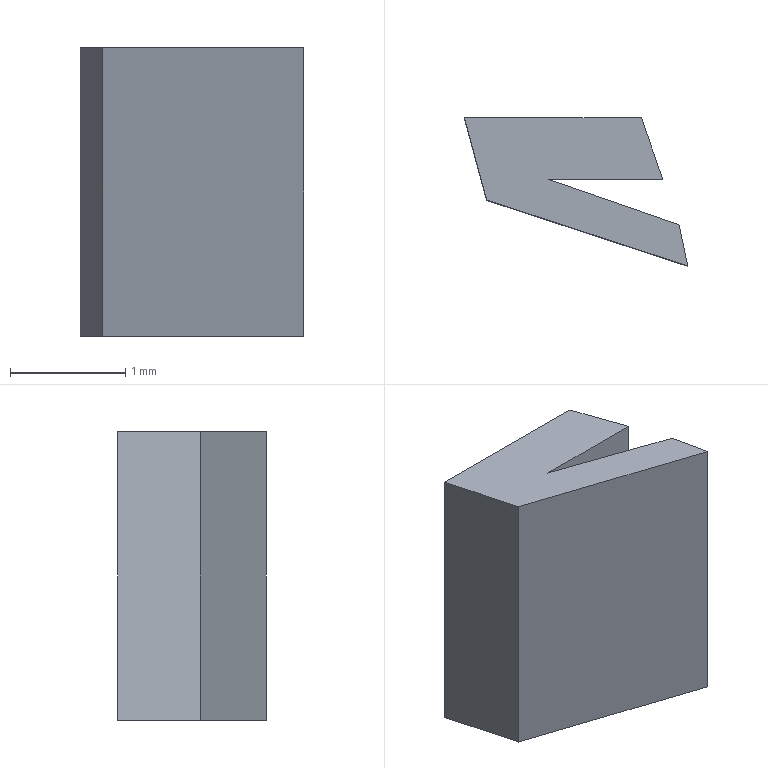Part | STEP file | lll_id1086_x_t | 1 solid | 9 faces | box 1.938 x 1.285 x 2.5 mm | volume 3.455 mm3 | plane 9
STEP:
#1=CARTESIAN_POINT('',(385.109,-124.499,2.35));
#2=VERTEX_POINT('',#1);
#3=CARTESIAN_POINT('',(385.184,-124.857,2.35));
#4=VERTEX_POINT('',#3);
#5=CARTESIAN_POINT('',(385.109,-124.499,2.35));
#6=DIRECTION('',(0.2057,-0.9786,0.));
#7=VECTOR('',#6,1.);
#8=LINE('',#5,#7);
#9=EDGE_CURVE('',#2,#4,#8,.T.);
#10=ORIENTED_EDGE('',*,*,#9,.T.);
#11=CARTESIAN_POINT('',(385.184,-124.857,-0.15));
#12=VERTEX_POINT('',#11);
#13=CARTESIAN_POINT('',(385.184,-124.857,-0.15));
#14=DIRECTION('',(0.,0.,1.));
#15=VECTOR('',#14,1.);
#16=LINE('',#13,#15);
#17=EDGE_CURVE('',#12,#4,#16,.T.);
#18=ORIENTED_EDGE('',*,*,#17,.F.);
#19=CARTESIAN_POINT('',(385.109,-124.499,-0.15));
#20=VERTEX_POINT('',#19);
#21=CARTESIAN_POINT('',(385.109,-124.499,-0.15));
#22=DIRECTION('',(0.2057,-0.9786,0.));
#23=VECTOR('',#22,1.);
#24=LINE('',#21,#23);
#25=EDGE_CURVE('',#20,#12,#24,.T.);
#26=ORIENTED_EDGE('',*,*,#25,.F.);
#27=CARTESIAN_POINT('',(385.109,-124.499,-0.15));
#28=DIRECTION('',(0.,0.,1.));
#29=VECTOR('',#28,1.);
#30=LINE('',#27,#29);
#31=EDGE_CURVE('',#20,#2,#30,.T.);
#32=ORIENTED_EDGE('',*,*,#31,.T.);
#33=EDGE_LOOP('',(#10,#18,#26,#32));
#34=FACE_OUTER_BOUND('',#33,.T.);
#35=CARTESIAN_POINT('',(385.109,-124.499,-0.15));
#36=DIRECTION('',(-0.9786,-0.2057,0.));
#37=DIRECTION('',(-0.2057,0.9786,0.));
#38=AXIS2_PLACEMENT_3D('',#35,#36,#37);
#39=PLANE('',#38);
#40=ADVANCED_FACE('',(#34),#39,.F.);
#41=CARTESIAN_POINT('',(383.439,-124.285,2.35));
#42=VERTEX_POINT('',#41);
#43=CARTESIAN_POINT('',(385.184,-124.857,2.35));
#44=DIRECTION('',(-0.9503,0.3113,0.));
#45=VECTOR('',#44,1.);
#46=LINE('',#43,#45);
#47=EDGE_CURVE('',#4,#42,#46,.T.);
#48=ORIENTED_EDGE('',*,*,#47,.T.);
#49=CARTESIAN_POINT('',(383.439,-124.285,-0.15));
#50=VERTEX_POINT('',#49);
#51=CARTESIAN_POINT('',(383.439,-124.285,-0.15));
#52=DIRECTION('',(0.,0.,1.));
#53=VECTOR('',#52,1.);
#54=LINE('',#51,#53);
#55=EDGE_CURVE('',#50,#42,#54,.T.);
#56=ORIENTED_EDGE('',*,*,#55,.F.);
#57=CARTESIAN_POINT('',(385.184,-124.857,-0.15));
#58=DIRECTION('',(-0.9503,0.3113,0.));
#59=VECTOR('',#58,1.);
#60=LINE('',#57,#59);
#61=EDGE_CURVE('',#12,#50,#60,.T.);
#62=ORIENTED_EDGE('',*,*,#61,.F.);
#63=ORIENTED_EDGE('',*,*,#17,.T.);
#64=EDGE_LOOP('',(#48,#56,#62,#63));
#65=FACE_OUTER_BOUND('',#64,.T.);
#66=CARTESIAN_POINT('',(385.184,-124.857,-0.15));
#67=DIRECTION('',(0.3113,0.9503,0.));
#68=DIRECTION('',(0.9503,-0.3113,0.));
#69=AXIS2_PLACEMENT_3D('',#66,#67,#68);
#70=PLANE('',#69);
#71=ADVANCED_FACE('',(#65),#70,.F.);
#72=CARTESIAN_POINT('',(383.246,-123.572,2.35));
#73=VERTEX_POINT('',#72);
#74=CARTESIAN_POINT('',(383.439,-124.285,2.35));
#75=DIRECTION('',(-0.261,0.9653,0.));
#76=VECTOR('',#75,1.);
#77=LINE('',#74,#76);
#78=EDGE_CURVE('',#42,#73,#77,.T.);
#79=ORIENTED_EDGE('',*,*,#78,.T.);
#80=CARTESIAN_POINT('',(383.246,-123.572,-0.15));
#81=VERTEX_POINT('',#80);
#82=CARTESIAN_POINT('',(383.246,-123.572,-0.15));
#83=DIRECTION('',(0.,0.,1.));
#84=VECTOR('',#83,1.);
#85=LINE('',#82,#84);
#86=EDGE_CURVE('',#81,#73,#85,.T.);
#87=ORIENTED_EDGE('',*,*,#86,.F.);
#88=CARTESIAN_POINT('',(383.439,-124.285,-0.15));
#89=DIRECTION('',(-0.261,0.9653,0.));
#90=VECTOR('',#89,1.);
#91=LINE('',#88,#90);
#92=EDGE_CURVE('',#50,#81,#91,.T.);
#93=ORIENTED_EDGE('',*,*,#92,.F.);
#94=ORIENTED_EDGE('',*,*,#55,.T.);
#95=EDGE_LOOP('',(#79,#87,#93,#94));
#96=FACE_OUTER_BOUND('',#95,.T.);
#97=CARTESIAN_POINT('',(383.439,-124.285,-0.15));
#98=DIRECTION('',(0.9653,0.261,0.));
#99=DIRECTION('',(0.261,-0.9653,0.));
#100=AXIS2_PLACEMENT_3D('',#97,#98,#99);
#101=PLANE('',#100);
#102=ADVANCED_FACE('',(#96),#101,.F.);
#103=CARTESIAN_POINT('',(384.782,-123.572,2.35));
#104=VERTEX_POINT('',#103);
#105=CARTESIAN_POINT('',(383.246,-123.572,2.35));
#106=DIRECTION('',(1.,0.,0.));
#107=VECTOR('',#106,1.);
#108=LINE('',#105,#107);
#109=EDGE_CURVE('',#73,#104,#108,.T.);
#110=ORIENTED_EDGE('',*,*,#109,.T.);
#111=CARTESIAN_POINT('',(384.782,-123.572,-0.15));
#112=VERTEX_POINT('',#111);
#113=CARTESIAN_POINT('',(384.782,-123.572,-0.15));
#114=DIRECTION('',(0.,0.,1.));
#115=VECTOR('',#114,1.);
#116=LINE('',#113,#115);
#117=EDGE_CURVE('',#112,#104,#116,.T.);
#118=ORIENTED_EDGE('',*,*,#117,.F.);
#119=CARTESIAN_POINT('',(383.246,-123.572,-0.15));
#120=DIRECTION('',(1.,0.,0.));
#121=VECTOR('',#120,1.);
#122=LINE('',#119,#121);
#123=EDGE_CURVE('',#81,#112,#122,.T.);
#124=ORIENTED_EDGE('',*,*,#123,.F.);
#125=ORIENTED_EDGE('',*,*,#86,.T.);
#126=EDGE_LOOP('',(#110,#118,#124,#125));
#127=FACE_OUTER_BOUND('',#126,.T.);
#128=CARTESIAN_POINT('',(383.246,-123.572,-0.15));
#129=DIRECTION('',(0.,-1.,0.));
#130=DIRECTION('',(0.,0.,-1.));
#131=AXIS2_PLACEMENT_3D('',#128,#129,#130);
#132=PLANE('',#131);
#133=ADVANCED_FACE('',(#127),#132,.F.);
#134=CARTESIAN_POINT('',(384.969,-124.107,2.35));
#135=VERTEX_POINT('',#134);
#136=CARTESIAN_POINT('',(384.782,-123.572,2.35));
#137=DIRECTION('',(0.3299,-0.944,0.));
#138=VECTOR('',#137,1.);
#139=LINE('',#136,#138);
#140=EDGE_CURVE('',#104,#135,#139,.T.);
#141=ORIENTED_EDGE('',*,*,#140,.T.);
#142=CARTESIAN_POINT('',(384.969,-124.107,-0.15));
#143=VERTEX_POINT('',#142);
#144=CARTESIAN_POINT('',(384.969,-124.107,-0.15));
#145=DIRECTION('',(0.,0.,1.));
#146=VECTOR('',#145,1.);
#147=LINE('',#144,#146);
#148=EDGE_CURVE('',#143,#135,#147,.T.);
#149=ORIENTED_EDGE('',*,*,#148,.F.);
#150=CARTESIAN_POINT('',(384.782,-123.572,-0.15));
#151=DIRECTION('',(0.3299,-0.944,0.));
#152=VECTOR('',#151,1.);
#153=LINE('',#150,#152);
#154=EDGE_CURVE('',#112,#143,#153,.T.);
#155=ORIENTED_EDGE('',*,*,#154,.F.);
#156=ORIENTED_EDGE('',*,*,#117,.T.);
#157=EDGE_LOOP('',(#141,#149,#155,#156));
#158=FACE_OUTER_BOUND('',#157,.T.);
#159=CARTESIAN_POINT('',(384.782,-123.572,-0.15));
#160=DIRECTION('',(-0.944,-0.3299,0.));
#161=DIRECTION('',(-0.3299,0.944,0.));
#162=AXIS2_PLACEMENT_3D('',#159,#160,#161);
#163=PLANE('',#162);
#164=ADVANCED_FACE('',(#158),#163,.F.);
#165=CARTESIAN_POINT('',(383.975,-124.107,2.35));
#166=VERTEX_POINT('',#165);
#167=CARTESIAN_POINT('',(384.969,-124.107,2.35));
#168=DIRECTION('',(-1.,0.,0.));
#169=VECTOR('',#168,1.);
#170=LINE('',#167,#169);
#171=EDGE_CURVE('',#135,#166,#170,.T.);
#172=ORIENTED_EDGE('',*,*,#171,.T.);
#173=CARTESIAN_POINT('',(383.975,-124.107,-0.15));
#174=VERTEX_POINT('',#173);
#175=CARTESIAN_POINT('',(383.975,-124.107,-0.15));
#176=DIRECTION('',(0.,0.,1.));
#177=VECTOR('',#176,1.);
#178=LINE('',#175,#177);
#179=EDGE_CURVE('',#174,#166,#178,.T.);
#180=ORIENTED_EDGE('',*,*,#179,.F.);
#181=CARTESIAN_POINT('',(384.969,-124.107,-0.15));
#182=DIRECTION('',(-1.,0.,0.));
#183=VECTOR('',#182,1.);
#184=LINE('',#181,#183);
#185=EDGE_CURVE('',#143,#174,#184,.T.);
#186=ORIENTED_EDGE('',*,*,#185,.F.);
#187=ORIENTED_EDGE('',*,*,#148,.T.);
#188=EDGE_LOOP('',(#172,#180,#186,#187));
#189=FACE_OUTER_BOUND('',#188,.T.);
#190=CARTESIAN_POINT('',(384.969,-124.107,-0.15));
#191=DIRECTION('',(0.,1.,0.));
#192=DIRECTION('',(0.,0.,1.));
#193=AXIS2_PLACEMENT_3D('',#190,#191,#192);
#194=PLANE('',#193);
#195=ADVANCED_FACE('',(#189),#194,.F.);
#196=CARTESIAN_POINT('',(383.975,-124.107,2.35));
#197=DIRECTION('',(0.9449,-0.3274,0.));
#198=VECTOR('',#197,1.);
#199=LINE('',#196,#198);
#200=EDGE_CURVE('',#166,#2,#199,.T.);
#201=ORIENTED_EDGE('',*,*,#200,.T.);
#202=ORIENTED_EDGE('',*,*,#31,.F.);
#203=CARTESIAN_POINT('',(383.975,-124.107,-0.15));
#204=DIRECTION('',(0.9449,-0.3274,0.));
#205=VECTOR('',#204,1.);
#206=LINE('',#203,#205);
#207=EDGE_CURVE('',#174,#20,#206,.T.);
#208=ORIENTED_EDGE('',*,*,#207,.F.);
#209=ORIENTED_EDGE('',*,*,#179,.T.);
#210=EDGE_LOOP('',(#201,#202,#208,#209));
#211=FACE_OUTER_BOUND('',#210,.T.);
#212=CARTESIAN_POINT('',(383.975,-124.107,-0.15));
#213=DIRECTION('',(-0.3274,-0.9449,0.));
#214=DIRECTION('',(-0.9449,0.3274,0.));
#215=AXIS2_PLACEMENT_3D('',#212,#213,#214);
#216=PLANE('',#215);
#217=ADVANCED_FACE('',(#211),#216,.F.);
#218=ORIENTED_EDGE('',*,*,#25,.T.);
#219=ORIENTED_EDGE('',*,*,#61,.T.);
#220=ORIENTED_EDGE('',*,*,#92,.T.);
#221=ORIENTED_EDGE('',*,*,#123,.T.);
#222=ORIENTED_EDGE('',*,*,#154,.T.);
#223=ORIENTED_EDGE('',*,*,#185,.T.);
#224=ORIENTED_EDGE('',*,*,#207,.T.);
#225=EDGE_LOOP('',(#218,#219,#220,#221,#222,#223,#224));
#226=FACE_OUTER_BOUND('',#225,.T.);
#227=CARTESIAN_POINT('',(-2493.249,1.,-0.15));
#228=DIRECTION('',(0.,0.,1.));
#229=DIRECTION('',(1.,0.,0.));
#230=AXIS2_PLACEMENT_3D('',#227,#228,#229);
#231=PLANE('',#230);
#232=ADVANCED_FACE('',(#226),#231,.F.);
#233=ORIENTED_EDGE('',*,*,#9,.F.);
#234=ORIENTED_EDGE('',*,*,#200,.F.);
#235=ORIENTED_EDGE('',*,*,#171,.F.);
#236=ORIENTED_EDGE('',*,*,#140,.F.);
#237=ORIENTED_EDGE('',*,*,#109,.F.);
#238=ORIENTED_EDGE('',*,*,#78,.F.);
#239=ORIENTED_EDGE('',*,*,#47,.F.);
#240=EDGE_LOOP('',(#233,#234,#235,#236,#237,#238,#239));
#241=FACE_OUTER_BOUND('',#240,.T.);
#242=CARTESIAN_POINT('',(-2493.249,1.,2.35));
#243=DIRECTION('',(0.,0.,1.));
#244=DIRECTION('',(1.,0.,0.));
#245=AXIS2_PLACEMENT_3D('',#242,#243,#244);
#246=PLANE('',#245);
#247=ADVANCED_FACE('',(#241),#246,.T.);
#248=CLOSED_SHELL('',(#40,#71,#102,#133,#164,#195,#217,#232,#247));
#249=MANIFOLD_SOLID_BREP('',#248);
#250=(LENGTH_UNIT()NAMED_UNIT(*)SI_UNIT(.MILLI.,.METRE.));
#251=UNCERTAINTY_MEASURE_WITH_UNIT(LENGTH_MEASURE(0.00002),#250,'','');
#252=(NAMED_UNIT(*)PLANE_ANGLE_UNIT()SI_UNIT($,.RADIAN.));
#253=PLANE_ANGLE_MEASURE_WITH_UNIT(PLANE_ANGLE_MEASURE(0.01745),#252);
#254=DIMENSIONAL_EXPONENTS(0.,0.,0.,0.,0.,0.,0.);
#255=(CONVERSION_BASED_UNIT('DEGREE',#253)NAMED_UNIT(#254)PLANE_ANGLE_UNIT());
#256=(NAMED_UNIT(*)SI_UNIT($,.STERADIAN.)SOLID_ANGLE_UNIT());
#257=(GEOMETRIC_REPRESENTATION_CONTEXT(3)GLOBAL_UNCERTAINTY_ASSIGNED_CONTEXT((#251))GLOBAL_UNIT_ASSIGNED_CONTEXT((#250,#255,#256))REPRESENTATION_CONTEXT('',''));
#258=ADVANCED_BREP_SHAPE_REPRESENTATION('',(#249),#257);